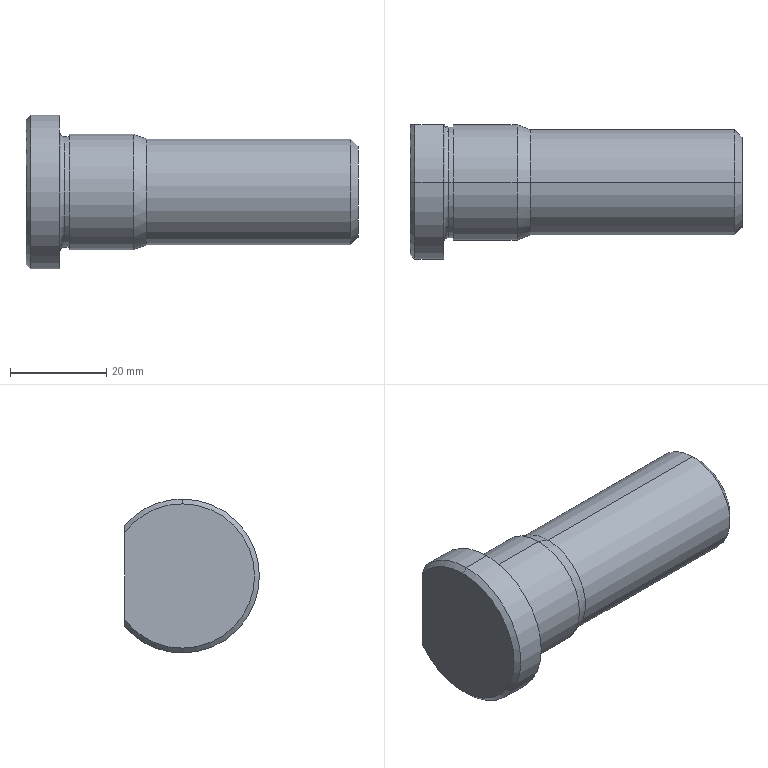Part | SolidWorks | features Chamfer 2, Fillet 1, ICE 1, Revolution 1 | 1 solid | 23 faces | box 69 x 28 x 32 mm | volume 29821 mm3 | cylinder 9 | cone 7 | plane 5 | torus 2 | commonest cylinder face diameters 32 x3 22 x2 23 x2 24 x2
STEP:
#1=CARTESIAN_POINT('',(69.,0.,-9.5));
#2=VERTEX_POINT('',#1);
#3=CARTESIAN_POINT('',(69.,0.,9.5));
#4=VERTEX_POINT('',#3);
#5=CARTESIAN_POINT('',(69.,0.,0.));
#6=DIRECTION('',(1.,0.,0.));
#7=DIRECTION('',(0.,0.,1.));
#8=AXIS2_PLACEMENT_3D('',#5,#6,#7);
#9=CIRCLE('',#8,9.5);
#10=EDGE_CURVE('',#2,#4,#9,.T.);
#11=ORIENTED_EDGE('',*,*,#10,.F.);
#12=CARTESIAN_POINT('',(67.5,0.,-11.));
#13=VERTEX_POINT('',#12);
#14=CARTESIAN_POINT('',(67.5,0.,-11.));
#15=DIRECTION('',(-0.7071,0.,-0.7071));
#16=VECTOR('',#15,1000.);
#17=LINE('',#14,#16);
#18=EDGE_CURVE('',#2,#13,#17,.T.);
#19=ORIENTED_EDGE('',*,*,#18,.T.);
#20=CARTESIAN_POINT('',(67.5,0.,11.));
#21=VERTEX_POINT('',#20);
#22=CARTESIAN_POINT('',(67.5,0.,0.));
#23=DIRECTION('',(-1.,0.,0.));
#24=DIRECTION('',(0.,0.,1.));
#25=AXIS2_PLACEMENT_3D('',#22,#23,#24);
#26=CIRCLE('',#25,11.);
#27=EDGE_CURVE('',#21,#13,#26,.T.);
#28=ORIENTED_EDGE('',*,*,#27,.F.);
#29=CARTESIAN_POINT('',(67.5,0.,11.));
#30=DIRECTION('',(-0.7071,0.,0.7071));
#31=VECTOR('',#30,1000.);
#32=LINE('',#29,#31);
#33=EDGE_CURVE('',#4,#21,#32,.T.);
#34=ORIENTED_EDGE('',*,*,#33,.F.);
#35=EDGE_LOOP('',(#11,#19,#28,#34));
#36=FACE_OUTER_BOUND('',#35,.T.);
#37=CARTESIAN_POINT('',(67.5,0.,0.));
#38=DIRECTION('',(-1.,0.,0.));
#39=DIRECTION('',(0.,0.,1.));
#40=AXIS2_PLACEMENT_3D('',#37,#38,#39);
#41=CONICAL_SURFACE('',#40,11.,0.7854);
#42=ADVANCED_FACE('',(#36),#41,.T.);
#43=ORIENTED_EDGE('',*,*,#27,.T.);
#44=CARTESIAN_POINT('',(25.,0.,-11.));
#45=VERTEX_POINT('',#44);
#46=CARTESIAN_POINT('',(-47.693,0.,-11.));
#47=DIRECTION('',(-1.,0.,0.));
#48=VECTOR('',#47,1000.);
#49=LINE('',#46,#48);
#50=EDGE_CURVE('',#13,#45,#49,.T.);
#51=ORIENTED_EDGE('',*,*,#50,.T.);
#52=CARTESIAN_POINT('',(25.,0.,11.));
#53=VERTEX_POINT('',#52);
#54=CARTESIAN_POINT('',(25.,0.,0.));
#55=DIRECTION('',(-1.,0.,0.));
#56=DIRECTION('',(0.,0.,1.));
#57=AXIS2_PLACEMENT_3D('',#54,#55,#56);
#58=CIRCLE('',#57,11.);
#59=EDGE_CURVE('',#53,#45,#58,.T.);
#60=ORIENTED_EDGE('',*,*,#59,.F.);
#61=CARTESIAN_POINT('',(-47.693,0.,11.));
#62=DIRECTION('',(-1.,0.,0.));
#63=VECTOR('',#62,1000.);
#64=LINE('',#61,#63);
#65=EDGE_CURVE('',#21,#53,#64,.T.);
#66=ORIENTED_EDGE('',*,*,#65,.F.);
#67=EDGE_LOOP('',(#43,#51,#60,#66));
#68=FACE_OUTER_BOUND('',#67,.T.);
#69=CARTESIAN_POINT('',(-47.693,0.,0.));
#70=DIRECTION('',(-1.,0.,0.));
#71=DIRECTION('',(0.,0.,1.));
#72=AXIS2_PLACEMENT_3D('',#69,#70,#71);
#73=CYLINDRICAL_SURFACE('',#72,11.);
#74=ADVANCED_FACE('',(#68),#73,.T.);
#75=ORIENTED_EDGE('',*,*,#59,.T.);
#76=CARTESIAN_POINT('',(22.253,0.,-12.));
#77=VERTEX_POINT('',#76);
#78=CARTESIAN_POINT('',(25.,0.,-11.));
#79=DIRECTION('',(-0.9397,0.,-0.342));
#80=VECTOR('',#79,1000.);
#81=LINE('',#78,#80);
#82=EDGE_CURVE('',#45,#77,#81,.T.);
#83=ORIENTED_EDGE('',*,*,#82,.T.);
#84=CARTESIAN_POINT('',(22.253,0.,12.));
#85=VERTEX_POINT('',#84);
#86=CARTESIAN_POINT('',(22.253,0.,0.));
#87=DIRECTION('',(-1.,0.,0.));
#88=DIRECTION('',(0.,0.,1.));
#89=AXIS2_PLACEMENT_3D('',#86,#87,#88);
#90=CIRCLE('',#89,12.);
#91=EDGE_CURVE('',#85,#77,#90,.T.);
#92=ORIENTED_EDGE('',*,*,#91,.F.);
#93=CARTESIAN_POINT('',(25.,0.,11.));
#94=DIRECTION('',(-0.9397,0.,0.342));
#95=VECTOR('',#94,1000.);
#96=LINE('',#93,#95);
#97=EDGE_CURVE('',#53,#85,#96,.T.);
#98=ORIENTED_EDGE('',*,*,#97,.F.);
#99=EDGE_LOOP('',(#75,#83,#92,#98));
#100=FACE_OUTER_BOUND('',#99,.T.);
#101=CARTESIAN_POINT('',(25.,0.,0.));
#102=DIRECTION('',(-1.,0.,0.));
#103=DIRECTION('',(0.,0.,1.));
#104=AXIS2_PLACEMENT_3D('',#101,#102,#103);
#105=CONICAL_SURFACE('',#104,11.,0.3491);
#106=ADVANCED_FACE('',(#100),#105,.T.);
#107=ORIENTED_EDGE('',*,*,#91,.T.);
#108=CARTESIAN_POINT('',(9.,0.,-12.));
#109=VERTEX_POINT('',#108);
#110=CARTESIAN_POINT('',(-47.693,0.,-12.));
#111=DIRECTION('',(-1.,0.,0.));
#112=VECTOR('',#111,1000.);
#113=LINE('',#110,#112);
#114=EDGE_CURVE('',#77,#109,#113,.T.);
#115=ORIENTED_EDGE('',*,*,#114,.T.);
#116=CARTESIAN_POINT('',(9.,0.,12.));
#117=VERTEX_POINT('',#116);
#118=CARTESIAN_POINT('',(9.,0.,0.));
#119=DIRECTION('',(-1.,0.,0.));
#120=DIRECTION('',(0.,0.,1.));
#121=AXIS2_PLACEMENT_3D('',#118,#119,#120);
#122=CIRCLE('',#121,12.);
#123=EDGE_CURVE('',#117,#109,#122,.T.);
#124=ORIENTED_EDGE('',*,*,#123,.F.);
#125=CARTESIAN_POINT('',(-47.693,0.,12.));
#126=DIRECTION('',(-1.,0.,0.));
#127=VECTOR('',#126,1000.);
#128=LINE('',#125,#127);
#129=EDGE_CURVE('',#85,#117,#128,.T.);
#130=ORIENTED_EDGE('',*,*,#129,.F.);
#131=EDGE_LOOP('',(#107,#115,#124,#130));
#132=FACE_OUTER_BOUND('',#131,.T.);
#133=CARTESIAN_POINT('',(-47.693,0.,0.));
#134=DIRECTION('',(-1.,0.,0.));
#135=DIRECTION('',(0.,0.,1.));
#136=AXIS2_PLACEMENT_3D('',#133,#134,#135);
#137=CYLINDRICAL_SURFACE('',#136,12.);
#138=ADVANCED_FACE('',(#132),#137,.T.);
#139=CARTESIAN_POINT('',(9.,0.,11.5));
#140=VERTEX_POINT('',#139);
#141=CARTESIAN_POINT('',(9.,0.,-11.5));
#142=VERTEX_POINT('',#141);
#143=CARTESIAN_POINT('',(9.,0.,0.));
#144=DIRECTION('',(-1.,0.,0.));
#145=DIRECTION('',(0.,0.,1.));
#146=AXIS2_PLACEMENT_3D('',#143,#144,#145);
#147=CIRCLE('',#146,11.5);
#148=EDGE_CURVE('',#140,#142,#147,.T.);
#149=ORIENTED_EDGE('',*,*,#148,.T.);
#150=CARTESIAN_POINT('',(8.,0.,-11.5));
#151=VERTEX_POINT('',#150);
#152=CARTESIAN_POINT('',(-47.693,0.,-11.5));
#153=DIRECTION('',(-1.,0.,0.));
#154=VECTOR('',#153,1000.);
#155=LINE('',#152,#154);
#156=EDGE_CURVE('',#142,#151,#155,.T.);
#157=ORIENTED_EDGE('',*,*,#156,.T.);
#158=CARTESIAN_POINT('',(8.,0.,11.5));
#159=VERTEX_POINT('',#158);
#160=CARTESIAN_POINT('',(8.,0.,0.));
#161=DIRECTION('',(1.,0.,0.));
#162=DIRECTION('',(0.,0.,1.));
#163=AXIS2_PLACEMENT_3D('',#160,#161,#162);
#164=CIRCLE('',#163,11.5);
#165=EDGE_CURVE('',#151,#159,#164,.T.);
#166=ORIENTED_EDGE('',*,*,#165,.T.);
#167=CARTESIAN_POINT('',(-47.693,0.,11.5));
#168=DIRECTION('',(-1.,0.,0.));
#169=VECTOR('',#168,1000.);
#170=LINE('',#167,#169);
#171=EDGE_CURVE('',#140,#159,#170,.T.);
#172=ORIENTED_EDGE('',*,*,#171,.F.);
#173=EDGE_LOOP('',(#149,#157,#166,#172));
#174=FACE_OUTER_BOUND('',#173,.T.);
#175=CARTESIAN_POINT('',(-47.693,0.,0.));
#176=DIRECTION('',(-1.,0.,0.));
#177=DIRECTION('',(0.,0.,1.));
#178=AXIS2_PLACEMENT_3D('',#175,#176,#177);
#179=CYLINDRICAL_SURFACE('',#178,11.5);
#180=ADVANCED_FACE('',(#174),#179,.T.);
#181=CARTESIAN_POINT('',(7.,0.,-12.5));
#182=VERTEX_POINT('',#181);
#183=CARTESIAN_POINT('',(7.,0.,12.5));
#184=VERTEX_POINT('',#183);
#185=CARTESIAN_POINT('',(7.,0.,0.));
#186=DIRECTION('',(-1.,0.,0.));
#187=DIRECTION('',(0.,0.,1.));
#188=AXIS2_PLACEMENT_3D('',#185,#186,#187);
#189=CIRCLE('',#188,12.5);
#190=EDGE_CURVE('',#182,#184,#189,.T.);
#191=ORIENTED_EDGE('',*,*,#190,.F.);
#192=CARTESIAN_POINT('',(8.,0.,-12.5));
#193=DIRECTION('',(0.,1.,0.));
#194=DIRECTION('',(0.,0.,1.));
#195=AXIS2_PLACEMENT_3D('',#192,#193,#194);
#196=CIRCLE('',#195,1.);
#197=EDGE_CURVE('',#182,#151,#196,.T.);
#198=ORIENTED_EDGE('',*,*,#197,.T.);
#199=CARTESIAN_POINT('',(8.,0.,0.));
#200=DIRECTION('',(1.,0.,0.));
#201=DIRECTION('',(0.,0.,1.));
#202=AXIS2_PLACEMENT_3D('',#199,#200,#201);
#203=CIRCLE('',#202,11.5);
#204=EDGE_CURVE('',#159,#151,#203,.T.);
#205=ORIENTED_EDGE('',*,*,#204,.F.);
#206=CARTESIAN_POINT('',(8.,0.,12.5));
#207=DIRECTION('',(0.,-1.,0.));
#208=DIRECTION('',(0.,0.,-1.));
#209=AXIS2_PLACEMENT_3D('',#206,#207,#208);
#210=CIRCLE('',#209,1.);
#211=EDGE_CURVE('',#184,#159,#210,.T.);
#212=ORIENTED_EDGE('',*,*,#211,.F.);
#213=EDGE_LOOP('',(#191,#198,#205,#212));
#214=FACE_OUTER_BOUND('',#213,.T.);
#215=CARTESIAN_POINT('',(8.,0.,0.));
#216=DIRECTION('',(-1.,0.,0.));
#217=DIRECTION('',(0.,0.,1.));
#218=AXIS2_PLACEMENT_3D('',#215,#216,#217);
#219=TOROIDAL_SURFACE('',#218,12.5,1.);
#220=ADVANCED_FACE('',(#214),#219,.F.);
#221=CARTESIAN_POINT('',(0.,0.,15.));
#222=VERTEX_POINT('',#221);
#223=CARTESIAN_POINT('',(0.,12.,9.));
#224=VERTEX_POINT('',#223);
#225=CARTESIAN_POINT('',(0.,0.,0.));
#226=DIRECTION('',(-1.,0.,0.));
#227=DIRECTION('',(0.,0.,-1.));
#228=AXIS2_PLACEMENT_3D('',#225,#226,#227);
#229=CIRCLE('',#228,15.);
#230=EDGE_CURVE('',#222,#224,#229,.T.);
#231=ORIENTED_EDGE('',*,*,#230,.F.);
#232=CARTESIAN_POINT('',(1.,0.,16.));
#233=VERTEX_POINT('',#232);
#234=CARTESIAN_POINT('',(0.,0.,15.));
#235=DIRECTION('',(0.7071,0.,0.7071));
#236=VECTOR('',#235,1000.);
#237=LINE('',#234,#236);
#238=EDGE_CURVE('',#222,#233,#237,.T.);
#239=ORIENTED_EDGE('',*,*,#238,.T.);
#240=CARTESIAN_POINT('',(1.,12.,10.583));
#241=VERTEX_POINT('',#240);
#242=CARTESIAN_POINT('',(1.,0.,0.));
#243=DIRECTION('',(1.,0.,0.));
#244=DIRECTION('',(0.,0.,-1.));
#245=AXIS2_PLACEMENT_3D('',#242,#243,#244);
#246=CIRCLE('',#245,16.);
#247=EDGE_CURVE('',#241,#233,#246,.T.);
#248=ORIENTED_EDGE('',*,*,#247,.F.);
#249=CARTESIAN_POINT('',(1.,12.,10.583));
#250=CARTESIAN_POINT('',(0.6557,12.,10.062));
#251=CARTESIAN_POINT('',(0.3213,12.,9.535));
#252=CARTESIAN_POINT('',(0.,12.,9.));
#253=B_SPLINE_CURVE_WITH_KNOTS('',3,(#249,#250,#251,#252),.UNSPECIFIED.,.F.,.F.,(4,4),(0.01632,0.0182),.UNSPECIFIED.);
#254=EDGE_CURVE('',#241,#224,#253,.T.);
#255=ORIENTED_EDGE('',*,*,#254,.T.);
#256=EDGE_LOOP('',(#231,#239,#248,#255));
#257=FACE_OUTER_BOUND('',#256,.T.);
#258=CARTESIAN_POINT('',(0.,0.,0.));
#259=DIRECTION('',(1.,0.,0.));
#260=DIRECTION('',(0.,0.,-1.));
#261=AXIS2_PLACEMENT_3D('',#258,#259,#260);
#262=CONICAL_SURFACE('',#261,15.,0.7854);
#263=ADVANCED_FACE('',(#257),#262,.T.);
#264=ORIENTED_EDGE('',*,*,#238,.F.);
#265=CARTESIAN_POINT('',(0.,0.,-15.));
#266=VERTEX_POINT('',#265);
#267=CARTESIAN_POINT('',(0.,0.,0.));
#268=DIRECTION('',(-1.,0.,0.));
#269=DIRECTION('',(0.,0.,-1.));
#270=AXIS2_PLACEMENT_3D('',#267,#268,#269);
#271=CIRCLE('',#270,15.);
#272=EDGE_CURVE('',#266,#222,#271,.T.);
#273=ORIENTED_EDGE('',*,*,#272,.F.);
#274=CARTESIAN_POINT('',(1.,0.,-16.));
#275=VERTEX_POINT('',#274);
#276=CARTESIAN_POINT('',(0.,0.,-15.));
#277=DIRECTION('',(0.7071,0.,-0.7071));
#278=VECTOR('',#277,1000.);
#279=LINE('',#276,#278);
#280=EDGE_CURVE('',#266,#275,#279,.T.);
#281=ORIENTED_EDGE('',*,*,#280,.T.);
#282=CARTESIAN_POINT('',(1.,0.,0.));
#283=DIRECTION('',(1.,0.,0.));
#284=DIRECTION('',(0.,0.,-1.));
#285=AXIS2_PLACEMENT_3D('',#282,#283,#284);
#286=CIRCLE('',#285,16.);
#287=EDGE_CURVE('',#233,#275,#286,.T.);
#288=ORIENTED_EDGE('',*,*,#287,.F.);
#289=EDGE_LOOP('',(#264,#273,#281,#288));
#290=FACE_OUTER_BOUND('',#289,.T.);
#291=CARTESIAN_POINT('',(0.,0.,0.));
#292=DIRECTION('',(1.,0.,0.));
#293=DIRECTION('',(0.,0.,-1.));
#294=AXIS2_PLACEMENT_3D('',#291,#292,#293);
#295=CONICAL_SURFACE('',#294,15.,0.7854);
#296=ADVANCED_FACE('',(#290),#295,.T.);
#297=CARTESIAN_POINT('',(7.,12.,-10.583));
#298=VERTEX_POINT('',#297);
#299=CARTESIAN_POINT('',(7.,0.,-16.));
#300=VERTEX_POINT('',#299);
#301=CARTESIAN_POINT('',(7.,0.,0.));
#302=DIRECTION('',(-1.,0.,0.));
#303=DIRECTION('',(0.,0.,1.));
#304=AXIS2_PLACEMENT_3D('',#301,#302,#303);
#305=CIRCLE('',#304,16.);
#306=EDGE_CURVE('',#298,#300,#305,.T.);
#307=ORIENTED_EDGE('',*,*,#306,.T.);
#308=CARTESIAN_POINT('',(-47.693,0.,-16.));
#309=DIRECTION('',(-1.,0.,0.));
#310=VECTOR('',#309,1000.);
#311=LINE('',#308,#310);
#312=EDGE_CURVE('',#300,#275,#311,.T.);
#313=ORIENTED_EDGE('',*,*,#312,.T.);
#314=CARTESIAN_POINT('',(1.,12.,-10.583));
#315=VERTEX_POINT('',#314);
#316=CARTESIAN_POINT('',(1.,0.,0.));
#317=DIRECTION('',(1.,0.,0.));
#318=DIRECTION('',(0.,0.,-1.));
#319=AXIS2_PLACEMENT_3D('',#316,#317,#318);
#320=CIRCLE('',#319,16.);
#321=EDGE_CURVE('',#275,#315,#320,.T.);
#322=ORIENTED_EDGE('',*,*,#321,.T.);
#323=CARTESIAN_POINT('',(8.,12.,-10.583));
#324=DIRECTION('',(-1.,0.,0.));
#325=VECTOR('',#324,1000.);
#326=LINE('',#323,#325);
#327=EDGE_CURVE('',#298,#315,#326,.T.);
#328=ORIENTED_EDGE('',*,*,#327,.F.);
#329=EDGE_LOOP('',(#307,#313,#322,#328));
#330=FACE_OUTER_BOUND('',#329,.T.);
#331=CARTESIAN_POINT('',(-47.693,0.,0.));
#332=DIRECTION('',(-1.,0.,0.));
#333=DIRECTION('',(0.,0.,1.));
#334=AXIS2_PLACEMENT_3D('',#331,#332,#333);
#335=CYLINDRICAL_SURFACE('',#334,16.);
#336=ADVANCED_FACE('',(#330),#335,.T.);
#337=ORIENTED_EDGE('',*,*,#312,.F.);
#338=CARTESIAN_POINT('',(7.,0.,16.));
#339=VERTEX_POINT('',#338);
#340=CARTESIAN_POINT('',(7.,0.,0.));
#341=DIRECTION('',(-1.,0.,0.));
#342=DIRECTION('',(0.,0.,1.));
#343=AXIS2_PLACEMENT_3D('',#340,#341,#342);
#344=CIRCLE('',#343,16.);
#345=EDGE_CURVE('',#300,#339,#344,.T.);
#346=ORIENTED_EDGE('',*,*,#345,.T.);
#347=CARTESIAN_POINT('',(-47.693,0.,16.));
#348=DIRECTION('',(-1.,0.,0.));
#349=VECTOR('',#348,1000.);
#350=LINE('',#347,#349);
#351=EDGE_CURVE('',#339,#233,#350,.T.);
#352=ORIENTED_EDGE('',*,*,#351,.T.);
#353=ORIENTED_EDGE('',*,*,#287,.T.);
#354=EDGE_LOOP('',(#337,#346,#352,#353));
#355=FACE_OUTER_BOUND('',#354,.T.);
#356=CARTESIAN_POINT('',(-47.693,0.,0.));
#357=DIRECTION('',(-1.,0.,0.));
#358=DIRECTION('',(0.,0.,1.));
#359=AXIS2_PLACEMENT_3D('',#356,#357,#358);
#360=CYLINDRICAL_SURFACE('',#359,16.);
#361=ADVANCED_FACE('',(#355),#360,.T.);
#362=CARTESIAN_POINT('',(0.,12.,-9.));
#363=VERTEX_POINT('',#362);
#364=CARTESIAN_POINT('',(0.,12.,10.583));
#365=DIRECTION('',(0.,0.,-1.));
#366=VECTOR('',#365,1000.);
#367=LINE('',#364,#366);
#368=EDGE_CURVE('',#224,#363,#367,.T.);
#369=ORIENTED_EDGE('',*,*,#368,.T.);
#370=CARTESIAN_POINT('',(0.,0.,0.));
#371=DIRECTION('',(-1.,0.,0.));
#372=DIRECTION('',(0.,0.,-1.));
#373=AXIS2_PLACEMENT_3D('',#370,#371,#372);
#374=CIRCLE('',#373,15.);
#375=EDGE_CURVE('',#363,#266,#374,.T.);
#376=ORIENTED_EDGE('',*,*,#375,.T.);
#377=ORIENTED_EDGE('',*,*,#272,.T.);
#378=ORIENTED_EDGE('',*,*,#230,.T.);
#379=EDGE_LOOP('',(#369,#376,#377,#378));
#380=FACE_OUTER_BOUND('',#379,.T.);
#381=CARTESIAN_POINT('',(0.,0.,0.));
#382=DIRECTION('',(1.,0.,0.));
#383=DIRECTION('',(0.,0.,-1.));
#384=AXIS2_PLACEMENT_3D('',#381,#382,#383);
#385=PLANE('',#384);
#386=ADVANCED_FACE('',(#380),#385,.F.);
#387=ORIENTED_EDGE('',*,*,#351,.F.);
#388=CARTESIAN_POINT('',(7.,12.,10.583));
#389=VERTEX_POINT('',#388);
#390=CARTESIAN_POINT('',(7.,0.,0.));
#391=DIRECTION('',(-1.,0.,0.));
#392=DIRECTION('',(0.,0.,1.));
#393=AXIS2_PLACEMENT_3D('',#390,#391,#392);
#394=CIRCLE('',#393,16.);
#395=EDGE_CURVE('',#339,#389,#394,.T.);
#396=ORIENTED_EDGE('',*,*,#395,.T.);
#397=CARTESIAN_POINT('',(8.,12.,10.583));
#398=DIRECTION('',(-1.,0.,0.));
#399=VECTOR('',#398,1000.);
#400=LINE('',#397,#399);
#401=EDGE_CURVE('',#389,#241,#400,.T.);
#402=ORIENTED_EDGE('',*,*,#401,.T.);
#403=ORIENTED_EDGE('',*,*,#247,.T.);
#404=EDGE_LOOP('',(#387,#396,#402,#403));
#405=FACE_OUTER_BOUND('',#404,.T.);
#406=CARTESIAN_POINT('',(-47.693,0.,0.));
#407=DIRECTION('',(-1.,0.,0.));
#408=DIRECTION('',(0.,0.,1.));
#409=AXIS2_PLACEMENT_3D('',#406,#407,#408);
#410=CYLINDRICAL_SURFACE('',#409,16.);
#411=ADVANCED_FACE('',(#405),#410,.T.);
#412=CARTESIAN_POINT('',(7.,12.,3.5));
#413=VERTEX_POINT('',#412);
#414=CARTESIAN_POINT('',(7.,12.,0.));
#415=DIRECTION('',(0.,0.,-1.));
#416=VECTOR('',#415,1000.);
#417=LINE('',#414,#416);
#418=EDGE_CURVE('',#389,#413,#417,.T.);
#419=ORIENTED_EDGE('',*,*,#418,.F.);
#420=ORIENTED_EDGE('',*,*,#395,.F.);
#421=ORIENTED_EDGE('',*,*,#345,.F.);
#422=ORIENTED_EDGE('',*,*,#306,.F.);
#423=CARTESIAN_POINT('',(7.,12.,-3.5));
#424=VERTEX_POINT('',#423);
#425=CARTESIAN_POINT('',(7.,12.,0.));
#426=DIRECTION('',(0.,0.,-1.));
#427=VECTOR('',#426,1000.);
#428=LINE('',#425,#427);
#429=EDGE_CURVE('',#424,#298,#428,.T.);
#430=ORIENTED_EDGE('',*,*,#429,.F.);
#431=CARTESIAN_POINT('',(7.,0.,0.));
#432=DIRECTION('',(-1.,0.,0.));
#433=DIRECTION('',(0.,0.,1.));
#434=AXIS2_PLACEMENT_3D('',#431,#432,#433);
#435=CIRCLE('',#434,12.5);
#436=EDGE_CURVE('',#424,#182,#435,.T.);
#437=ORIENTED_EDGE('',*,*,#436,.T.);
#438=ORIENTED_EDGE('',*,*,#190,.T.);
#439=CARTESIAN_POINT('',(7.,0.,0.));
#440=DIRECTION('',(-1.,0.,0.));
#441=DIRECTION('',(0.,0.,1.));
#442=AXIS2_PLACEMENT_3D('',#439,#440,#441);
#443=CIRCLE('',#442,12.5);
#444=EDGE_CURVE('',#184,#413,#443,.T.);
#445=ORIENTED_EDGE('',*,*,#444,.T.);
#446=EDGE_LOOP('',(#419,#420,#421,#422,#430,#437,#438,#445));
#447=FACE_OUTER_BOUND('',#446,.T.);
#448=CARTESIAN_POINT('',(7.,16.,0.));
#449=DIRECTION('',(-1.,0.,0.));
#450=DIRECTION('',(0.,0.,1.));
#451=AXIS2_PLACEMENT_3D('',#448,#449,#450);
#452=PLANE('',#451);
#453=ADVANCED_FACE('',(#447),#452,.F.);
#454=ORIENTED_EDGE('',*,*,#280,.F.);
#455=ORIENTED_EDGE('',*,*,#375,.F.);
#456=CARTESIAN_POINT('',(0.,12.,-9.));
#457=CARTESIAN_POINT('',(0.3209,12.,-9.535));
#458=CARTESIAN_POINT('',(0.6561,12.,-10.063));
#459=CARTESIAN_POINT('',(1.,12.,-10.583));
#460=B_SPLINE_CURVE_WITH_KNOTS('',3,(#456,#457,#458,#459),.UNSPECIFIED.,.F.,.F.,(4,4),(0.03741,0.03928),.UNSPECIFIED.);
#461=EDGE_CURVE('',#363,#315,#460,.T.);
#462=ORIENTED_EDGE('',*,*,#461,.T.);
#463=ORIENTED_EDGE('',*,*,#321,.F.);
#464=EDGE_LOOP('',(#454,#455,#462,#463));
#465=FACE_OUTER_BOUND('',#464,.T.);
#466=CARTESIAN_POINT('',(0.,0.,0.));
#467=DIRECTION('',(1.,0.,0.));
#468=DIRECTION('',(0.,0.,-1.));
#469=AXIS2_PLACEMENT_3D('',#466,#467,#468);
#470=CONICAL_SURFACE('',#469,15.,0.7854);
#471=ADVANCED_FACE('',(#465),#470,.T.);
#472=ORIENTED_EDGE('',*,*,#197,.F.);
#473=ORIENTED_EDGE('',*,*,#436,.F.);
#474=CARTESIAN_POINT('',(7.,12.,3.5));
#475=CARTESIAN_POINT('',(7.,12.,2.92));
#476=CARTESIAN_POINT('',(7.038,12.,2.339));
#477=CARTESIAN_POINT('',(7.105,12.,1.178));
#478=CARTESIAN_POINT('',(7.134,12.,0.5979));
#479=CARTESIAN_POINT('',(7.134,12.,-0.1286));
#480=CARTESIAN_POINT('',(7.133,12.,-0.2766));
#481=CARTESIAN_POINT('',(7.127,12.,-0.5699));
#482=CARTESIAN_POINT('',(7.122,12.,-0.7165));
#483=CARTESIAN_POINT('',(7.106,12.,-1.156));
#484=CARTESIAN_POINT('',(7.09,12.,-1.449));
#485=CARTESIAN_POINT('',(7.039,12.,-2.328));
#486=CARTESIAN_POINT('',(7.,12.,-2.913));
#487=CARTESIAN_POINT('',(7.,12.,-3.5));
#488=B_SPLINE_CURVE_WITH_KNOTS('',3,(#474,#475,#476,#477,#478,#479,#480,#481,#482,#483,#484,#485,#486,#487),.UNSPECIFIED.,.F.,.F.,(4,2,2,2,2,2,4),(0.02287,0.02463,0.02639,0.02683,0.02727,0.02814,0.0299),.UNSPECIFIED.);
#489=EDGE_CURVE('',#413,#424,#488,.T.);
#490=ORIENTED_EDGE('',*,*,#489,.F.);
#491=ORIENTED_EDGE('',*,*,#444,.F.);
#492=ORIENTED_EDGE('',*,*,#211,.T.);
#493=ORIENTED_EDGE('',*,*,#165,.F.);
#494=EDGE_LOOP('',(#472,#473,#490,#491,#492,#493));
#495=FACE_OUTER_BOUND('',#494,.T.);
#496=CARTESIAN_POINT('',(8.,0.,0.));
#497=DIRECTION('',(-1.,0.,0.));
#498=DIRECTION('',(0.,0.,1.));
#499=AXIS2_PLACEMENT_3D('',#496,#497,#498);
#500=TOROIDAL_SURFACE('',#499,12.5,1.);
#501=ADVANCED_FACE('',(#495),#500,.F.);
#502=ORIENTED_EDGE('',*,*,#156,.F.);
#503=CARTESIAN_POINT('',(9.,0.,0.));
#504=DIRECTION('',(-1.,0.,0.));
#505=DIRECTION('',(0.,0.,1.));
#506=AXIS2_PLACEMENT_3D('',#503,#504,#505);
#507=CIRCLE('',#506,11.5);
#508=EDGE_CURVE('',#142,#140,#507,.T.);
#509=ORIENTED_EDGE('',*,*,#508,.T.);
#510=ORIENTED_EDGE('',*,*,#171,.T.);
#511=ORIENTED_EDGE('',*,*,#204,.T.);
#512=EDGE_LOOP('',(#502,#509,#510,#511));
#513=FACE_OUTER_BOUND('',#512,.T.);
#514=CARTESIAN_POINT('',(-47.693,0.,0.));
#515=DIRECTION('',(-1.,0.,0.));
#516=DIRECTION('',(0.,0.,1.));
#517=AXIS2_PLACEMENT_3D('',#514,#515,#516);
#518=CYLINDRICAL_SURFACE('',#517,11.5);
#519=ADVANCED_FACE('',(#513),#518,.T.);
#520=ORIENTED_EDGE('',*,*,#148,.F.);
#521=ORIENTED_EDGE('',*,*,#508,.F.);
#522=EDGE_LOOP('',(#520,#521));
#523=FACE_BOUND('',#522,.T.);
#524=ORIENTED_EDGE('',*,*,#123,.T.);
#525=CARTESIAN_POINT('',(9.,0.,0.));
#526=DIRECTION('',(-1.,0.,0.));
#527=DIRECTION('',(0.,0.,1.));
#528=AXIS2_PLACEMENT_3D('',#525,#526,#527);
#529=CIRCLE('',#528,12.);
#530=EDGE_CURVE('',#109,#117,#529,.T.);
#531=ORIENTED_EDGE('',*,*,#530,.T.);
#532=EDGE_LOOP('',(#524,#531));
#533=FACE_OUTER_BOUND('',#532,.T.);
#534=CARTESIAN_POINT('',(9.,11.5,0.));
#535=DIRECTION('',(1.,0.,0.));
#536=DIRECTION('',(0.,0.,-1.));
#537=AXIS2_PLACEMENT_3D('',#534,#535,#536);
#538=PLANE('',#537);
#539=ADVANCED_FACE('',(#523,#533),#538,.F.);
#540=ORIENTED_EDGE('',*,*,#114,.F.);
#541=CARTESIAN_POINT('',(22.253,0.,0.));
#542=DIRECTION('',(-1.,0.,0.));
#543=DIRECTION('',(0.,0.,1.));
#544=AXIS2_PLACEMENT_3D('',#541,#542,#543);
#545=CIRCLE('',#544,12.);
#546=EDGE_CURVE('',#77,#85,#545,.T.);
#547=ORIENTED_EDGE('',*,*,#546,.T.);
#548=ORIENTED_EDGE('',*,*,#129,.T.);
#549=ORIENTED_EDGE('',*,*,#530,.F.);
#550=EDGE_LOOP('',(#540,#547,#548,#549));
#551=FACE_OUTER_BOUND('',#550,.T.);
#552=CARTESIAN_POINT('',(-47.693,0.,0.));
#553=DIRECTION('',(-1.,0.,0.));
#554=DIRECTION('',(0.,0.,1.));
#555=AXIS2_PLACEMENT_3D('',#552,#553,#554);
#556=CYLINDRICAL_SURFACE('',#555,12.);
#557=ADVANCED_FACE('',(#551),#556,.T.);
#558=ORIENTED_EDGE('',*,*,#82,.F.);
#559=CARTESIAN_POINT('',(25.,0.,0.));
#560=DIRECTION('',(-1.,0.,0.));
#561=DIRECTION('',(0.,0.,1.));
#562=AXIS2_PLACEMENT_3D('',#559,#560,#561);
#563=CIRCLE('',#562,11.);
#564=EDGE_CURVE('',#45,#53,#563,.T.);
#565=ORIENTED_EDGE('',*,*,#564,.T.);
#566=ORIENTED_EDGE('',*,*,#97,.T.);
#567=ORIENTED_EDGE('',*,*,#546,.F.);
#568=EDGE_LOOP('',(#558,#565,#566,#567));
#569=FACE_OUTER_BOUND('',#568,.T.);
#570=CARTESIAN_POINT('',(25.,0.,0.));
#571=DIRECTION('',(-1.,0.,0.));
#572=DIRECTION('',(0.,0.,1.));
#573=AXIS2_PLACEMENT_3D('',#570,#571,#572);
#574=CONICAL_SURFACE('',#573,11.,0.3491);
#575=ADVANCED_FACE('',(#569),#574,.T.);
#576=ORIENTED_EDGE('',*,*,#50,.F.);
#577=CARTESIAN_POINT('',(67.5,0.,0.));
#578=DIRECTION('',(-1.,0.,0.));
#579=DIRECTION('',(0.,0.,1.));
#580=AXIS2_PLACEMENT_3D('',#577,#578,#579);
#581=CIRCLE('',#580,11.);
#582=EDGE_CURVE('',#13,#21,#581,.T.);
#583=ORIENTED_EDGE('',*,*,#582,.T.);
#584=ORIENTED_EDGE('',*,*,#65,.T.);
#585=ORIENTED_EDGE('',*,*,#564,.F.);
#586=EDGE_LOOP('',(#576,#583,#584,#585));
#587=FACE_OUTER_BOUND('',#586,.T.);
#588=CARTESIAN_POINT('',(-47.693,0.,0.));
#589=DIRECTION('',(-1.,0.,0.));
#590=DIRECTION('',(0.,0.,1.));
#591=AXIS2_PLACEMENT_3D('',#588,#589,#590);
#592=CYLINDRICAL_SURFACE('',#591,11.);
#593=ADVANCED_FACE('',(#587),#592,.T.);
#594=CARTESIAN_POINT('',(69.,0.,0.));
#595=DIRECTION('',(1.,0.,0.));
#596=DIRECTION('',(0.,0.,1.));
#597=AXIS2_PLACEMENT_3D('',#594,#595,#596);
#598=CIRCLE('',#597,9.5);
#599=EDGE_CURVE('',#4,#2,#598,.T.);
#600=ORIENTED_EDGE('',*,*,#599,.T.);
#601=ORIENTED_EDGE('',*,*,#10,.T.);
#602=EDGE_LOOP('',(#600,#601));
#603=FACE_OUTER_BOUND('',#602,.T.);
#604=CARTESIAN_POINT('',(69.,11.,0.));
#605=DIRECTION('',(-1.,0.,0.));
#606=DIRECTION('',(0.,0.,1.));
#607=AXIS2_PLACEMENT_3D('',#604,#605,#606);
#608=PLANE('',#607);
#609=ADVANCED_FACE('',(#603),#608,.F.);
#610=ORIENTED_EDGE('',*,*,#18,.F.);
#611=ORIENTED_EDGE('',*,*,#599,.F.);
#612=ORIENTED_EDGE('',*,*,#33,.T.);
#613=ORIENTED_EDGE('',*,*,#582,.F.);
#614=EDGE_LOOP('',(#610,#611,#612,#613));
#615=FACE_OUTER_BOUND('',#614,.T.);
#616=CARTESIAN_POINT('',(67.5,0.,0.));
#617=DIRECTION('',(-1.,0.,0.));
#618=DIRECTION('',(0.,0.,1.));
#619=AXIS2_PLACEMENT_3D('',#616,#617,#618);
#620=CONICAL_SURFACE('',#619,11.,0.7854);
#621=ADVANCED_FACE('',(#615),#620,.T.);
#622=ORIENTED_EDGE('',*,*,#401,.F.);
#623=ORIENTED_EDGE('',*,*,#418,.T.);
#624=ORIENTED_EDGE('',*,*,#489,.T.);
#625=ORIENTED_EDGE('',*,*,#429,.T.);
#626=ORIENTED_EDGE('',*,*,#327,.T.);
#627=ORIENTED_EDGE('',*,*,#461,.F.);
#628=ORIENTED_EDGE('',*,*,#368,.F.);
#629=ORIENTED_EDGE('',*,*,#254,.F.);
#630=EDGE_LOOP('',(#622,#623,#624,#625,#626,#627,#628,#629));
#631=FACE_OUTER_BOUND('',#630,.T.);
#632=CARTESIAN_POINT('',(8.,12.,10.583));
#633=DIRECTION('',(0.,1.,0.));
#634=DIRECTION('',(0.,0.,1.));
#635=AXIS2_PLACEMENT_3D('',#632,#633,#634);
#636=PLANE('',#635);
#637=ADVANCED_FACE('',(#631),#636,.T.);
#638=CLOSED_SHELL('',(#42,#74,#106,#138,#180,#220,#263,#296,#336,#361,#386,#411,#453,#471,#501,#519,#539,#557,#575,#593,#609,#621,#637));
#639=MANIFOLD_SOLID_BREP('',#638);
#640=CARTESIAN_POINT('',(0.,0.,0.));
#641=DIRECTION('',(0.,0.,1.));
#642=DIRECTION('',(1.,0.,0.));
#643=AXIS2_PLACEMENT_3D('',#640,#641,#642);
#644=(LENGTH_UNIT()NAMED_UNIT(*)SI_UNIT(.MILLI.,.METRE.));
#645=UNCERTAINTY_MEASURE_WITH_UNIT(LENGTH_MEASURE(0.00001),#644,'','');
#646=(NAMED_UNIT(*)PLANE_ANGLE_UNIT()SI_UNIT($,.RADIAN.));
#647=(NAMED_UNIT(*)SI_UNIT($,.STERADIAN.)SOLID_ANGLE_UNIT());
#648=(GEOMETRIC_REPRESENTATION_CONTEXT(3)GLOBAL_UNCERTAINTY_ASSIGNED_CONTEXT((#645))GLOBAL_UNIT_ASSIGNED_CONTEXT((#644,#646,#647))REPRESENTATION_CONTEXT('',''));
#649=ADVANCED_BREP_SHAPE_REPRESENTATION('',(#639,#643),#648);